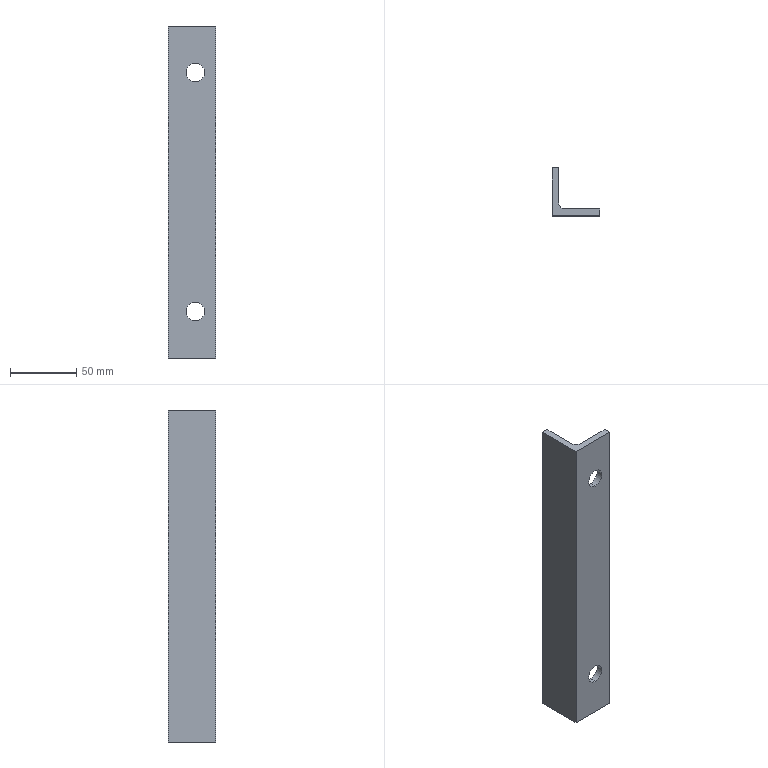Part | NX | features BREP 1 | 1 solid | 13 faces | box 36 x 36 x 250 mm | volume 83297 mm3 | plane 8 | cylinder 5 | commonest cylinder face diameters 14 x4 9 x1
STEP:
#1=CARTESIAN_POINT('',(20.5,0.,-97.));
#2=VERTEX_POINT('',#1);
#3=CARTESIAN_POINT('',(20.5,0.,-83.));
#4=VERTEX_POINT('',#3);
#5=CARTESIAN_POINT('',(20.5,0.,-90.));
#6=DIRECTION('',(0.,1.,0.));
#7=DIRECTION('',(0.,0.,-1.));
#8=AXIS2_PLACEMENT_3D('',#5,#6,#7);
#9=CIRCLE('',#8,7.);
#10=EDGE_CURVE('',#2,#4,#9,.T.);
#11=ORIENTED_EDGE('',*,*,#10,.F.);
#12=CARTESIAN_POINT('',(20.5,5.,-97.));
#13=VERTEX_POINT('',#12);
#14=CARTESIAN_POINT('',(20.5,0.,-97.));
#15=DIRECTION('',(0.,1.,0.));
#16=VECTOR('',#15,1000.);
#17=LINE('',#14,#16);
#18=EDGE_CURVE('',#2,#13,#17,.T.);
#19=ORIENTED_EDGE('',*,*,#18,.T.);
#20=CARTESIAN_POINT('',(20.5,5.,-83.));
#21=VERTEX_POINT('',#20);
#22=CARTESIAN_POINT('',(20.5,5.,-90.));
#23=DIRECTION('',(0.,1.,0.));
#24=DIRECTION('',(0.,0.,-1.));
#25=AXIS2_PLACEMENT_3D('',#22,#23,#24);
#26=CIRCLE('',#25,7.);
#27=EDGE_CURVE('',#13,#21,#26,.T.);
#28=ORIENTED_EDGE('',*,*,#27,.T.);
#29=CARTESIAN_POINT('',(20.5,0.,-83.));
#30=DIRECTION('',(0.,1.,0.));
#31=VECTOR('',#30,1000.);
#32=LINE('',#29,#31);
#33=EDGE_CURVE('',#4,#21,#32,.T.);
#34=ORIENTED_EDGE('',*,*,#33,.F.);
#35=EDGE_LOOP('',(#11,#19,#28,#34));
#36=FACE_BOUND('',#35,.T.);
#37=CARTESIAN_POINT('',(20.5,0.,-90.));
#38=DIRECTION('',(0.,1.,0.));
#39=DIRECTION('',(0.,0.,-1.));
#40=AXIS2_PLACEMENT_3D('',#37,#38,#39);
#41=CYLINDRICAL_SURFACE('',#40,7.);
#42=ADVANCED_FACE('',(#36),#41,.F.);
#43=CARTESIAN_POINT('',(20.5,0.,83.));
#44=VERTEX_POINT('',#43);
#45=CARTESIAN_POINT('',(20.5,0.,97.));
#46=VERTEX_POINT('',#45);
#47=CARTESIAN_POINT('',(20.5,0.,90.));
#48=DIRECTION('',(0.,1.,0.));
#49=DIRECTION('',(0.,0.,1.));
#50=AXIS2_PLACEMENT_3D('',#47,#48,#49);
#51=CIRCLE('',#50,7.);
#52=EDGE_CURVE('',#44,#46,#51,.T.);
#53=ORIENTED_EDGE('',*,*,#52,.F.);
#54=CARTESIAN_POINT('',(20.5,5.,83.));
#55=VERTEX_POINT('',#54);
#56=CARTESIAN_POINT('',(20.5,0.,83.));
#57=DIRECTION('',(0.,1.,0.));
#58=VECTOR('',#57,1000.);
#59=LINE('',#56,#58);
#60=EDGE_CURVE('',#44,#55,#59,.T.);
#61=ORIENTED_EDGE('',*,*,#60,.T.);
#62=CARTESIAN_POINT('',(20.5,5.,97.));
#63=VERTEX_POINT('',#62);
#64=CARTESIAN_POINT('',(20.5,5.,90.));
#65=DIRECTION('',(0.,1.,0.));
#66=DIRECTION('',(0.,0.,1.));
#67=AXIS2_PLACEMENT_3D('',#64,#65,#66);
#68=CIRCLE('',#67,7.);
#69=EDGE_CURVE('',#55,#63,#68,.T.);
#70=ORIENTED_EDGE('',*,*,#69,.T.);
#71=CARTESIAN_POINT('',(20.5,0.,97.));
#72=DIRECTION('',(0.,1.,0.));
#73=VECTOR('',#72,1000.);
#74=LINE('',#71,#73);
#75=EDGE_CURVE('',#46,#63,#74,.T.);
#76=ORIENTED_EDGE('',*,*,#75,.F.);
#77=EDGE_LOOP('',(#53,#61,#70,#76));
#78=FACE_BOUND('',#77,.T.);
#79=CARTESIAN_POINT('',(20.5,0.,90.));
#80=DIRECTION('',(0.,1.,0.));
#81=DIRECTION('',(0.,0.,-1.));
#82=AXIS2_PLACEMENT_3D('',#79,#80,#81);
#83=CYLINDRICAL_SURFACE('',#82,7.);
#84=ADVANCED_FACE('',(#78),#83,.F.);
#85=CARTESIAN_POINT('',(36.,0.,-125.));
#86=VERTEX_POINT('',#85);
#87=CARTESIAN_POINT('',(36.,5.,-125.));
#88=VERTEX_POINT('',#87);
#89=CARTESIAN_POINT('',(36.,5.,-125.));
#90=DIRECTION('',(0.,1.,0.));
#91=VECTOR('',#90,1000.);
#92=LINE('',#89,#91);
#93=EDGE_CURVE('',#86,#88,#92,.T.);
#94=ORIENTED_EDGE('',*,*,#93,.T.);
#95=CARTESIAN_POINT('',(36.,5.,125.));
#96=VERTEX_POINT('',#95);
#97=CARTESIAN_POINT('',(36.,5.,125.));
#98=DIRECTION('',(0.,0.,-1.));
#99=VECTOR('',#98,1000.);
#100=LINE('',#97,#99);
#101=EDGE_CURVE('',#96,#88,#100,.T.);
#102=ORIENTED_EDGE('',*,*,#101,.F.);
#103=CARTESIAN_POINT('',(36.,0.,125.));
#104=VERTEX_POINT('',#103);
#105=CARTESIAN_POINT('',(36.,5.,125.));
#106=DIRECTION('',(0.,1.,0.));
#107=VECTOR('',#106,1000.);
#108=LINE('',#105,#107);
#109=EDGE_CURVE('',#104,#96,#108,.T.);
#110=ORIENTED_EDGE('',*,*,#109,.F.);
#111=CARTESIAN_POINT('',(36.,0.,125.));
#112=DIRECTION('',(0.,0.,-1.));
#113=VECTOR('',#112,1000.);
#114=LINE('',#111,#113);
#115=EDGE_CURVE('',#104,#86,#114,.T.);
#116=ORIENTED_EDGE('',*,*,#115,.T.);
#117=EDGE_LOOP('',(#94,#102,#110,#116));
#118=FACE_BOUND('',#117,.T.);
#119=CARTESIAN_POINT('',(36.,5.,125.));
#120=DIRECTION('',(-1.,0.,0.));
#121=DIRECTION('',(0.,0.,-1.));
#122=AXIS2_PLACEMENT_3D('',#119,#120,#121);
#123=PLANE('',#122);
#124=ADVANCED_FACE('',(#118),#123,.F.);
#125=CARTESIAN_POINT('',(20.5,5.,-90.));
#126=DIRECTION('',(0.,1.,0.));
#127=DIRECTION('',(0.,0.,-1.));
#128=AXIS2_PLACEMENT_3D('',#125,#126,#127);
#129=CIRCLE('',#128,7.);
#130=EDGE_CURVE('',#21,#13,#129,.T.);
#131=ORIENTED_EDGE('',*,*,#130,.F.);
#132=ORIENTED_EDGE('',*,*,#27,.F.);
#133=EDGE_LOOP('',(#131,#132));
#134=FACE_BOUND('',#133,.T.);
#135=CARTESIAN_POINT('',(20.5,5.,90.));
#136=DIRECTION('',(0.,1.,0.));
#137=DIRECTION('',(0.,0.,1.));
#138=AXIS2_PLACEMENT_3D('',#135,#136,#137);
#139=CIRCLE('',#138,7.);
#140=EDGE_CURVE('',#63,#55,#139,.T.);
#141=ORIENTED_EDGE('',*,*,#140,.F.);
#142=ORIENTED_EDGE('',*,*,#69,.F.);
#143=EDGE_LOOP('',(#141,#142));
#144=FACE_BOUND('',#143,.T.);
#145=CARTESIAN_POINT('',(9.5,5.,-125.));
#146=VERTEX_POINT('',#145);
#147=CARTESIAN_POINT('',(9.5,5.,-125.));
#148=DIRECTION('',(-1.,0.,0.));
#149=VECTOR('',#148,1000.);
#150=LINE('',#147,#149);
#151=EDGE_CURVE('',#88,#146,#150,.T.);
#152=ORIENTED_EDGE('',*,*,#151,.T.);
#153=CARTESIAN_POINT('',(9.5,5.,125.));
#154=VERTEX_POINT('',#153);
#155=CARTESIAN_POINT('',(9.5,5.,125.));
#156=DIRECTION('',(0.,0.,-1.));
#157=VECTOR('',#156,1000.);
#158=LINE('',#155,#157);
#159=EDGE_CURVE('',#154,#146,#158,.T.);
#160=ORIENTED_EDGE('',*,*,#159,.F.);
#161=CARTESIAN_POINT('',(9.5,5.,125.));
#162=DIRECTION('',(-1.,0.,0.));
#163=VECTOR('',#162,1000.);
#164=LINE('',#161,#163);
#165=EDGE_CURVE('',#96,#154,#164,.T.);
#166=ORIENTED_EDGE('',*,*,#165,.F.);
#167=ORIENTED_EDGE('',*,*,#101,.T.);
#168=EDGE_LOOP('',(#152,#160,#166,#167));
#169=FACE_BOUND('',#168,.T.);
#170=CARTESIAN_POINT('',(9.5,5.,125.));
#171=DIRECTION('',(0.,-1.,0.));
#172=DIRECTION('',(0.,0.,1.));
#173=AXIS2_PLACEMENT_3D('',#170,#171,#172);
#174=PLANE('',#173);
#175=ADVANCED_FACE('',(#134,#144,#169),#174,.F.);
#176=CARTESIAN_POINT('',(5.,9.5,-125.));
#177=VERTEX_POINT('',#176);
#178=CARTESIAN_POINT('',(9.5,9.5,-125.));
#179=DIRECTION('',(0.,0.,-1.));
#180=DIRECTION('',(1.,0.,0.));
#181=AXIS2_PLACEMENT_3D('',#178,#179,#180);
#182=CIRCLE('',#181,4.5);
#183=EDGE_CURVE('',#146,#177,#182,.T.);
#184=ORIENTED_EDGE('',*,*,#183,.T.);
#185=CARTESIAN_POINT('',(5.,9.5,125.));
#186=VERTEX_POINT('',#185);
#187=CARTESIAN_POINT('',(5.,9.5,125.));
#188=DIRECTION('',(0.,0.,-1.));
#189=VECTOR('',#188,1000.);
#190=LINE('',#187,#189);
#191=EDGE_CURVE('',#186,#177,#190,.T.);
#192=ORIENTED_EDGE('',*,*,#191,.F.);
#193=CARTESIAN_POINT('',(9.5,9.5,125.));
#194=DIRECTION('',(0.,0.,-1.));
#195=DIRECTION('',(1.,0.,0.));
#196=AXIS2_PLACEMENT_3D('',#193,#194,#195);
#197=CIRCLE('',#196,4.5);
#198=EDGE_CURVE('',#154,#186,#197,.T.);
#199=ORIENTED_EDGE('',*,*,#198,.F.);
#200=ORIENTED_EDGE('',*,*,#159,.T.);
#201=EDGE_LOOP('',(#184,#192,#199,#200));
#202=FACE_BOUND('',#201,.T.);
#203=CARTESIAN_POINT('',(9.5,9.5,125.));
#204=DIRECTION('',(0.,0.,-1.));
#205=DIRECTION('',(1.,0.,0.));
#206=AXIS2_PLACEMENT_3D('',#203,#204,#205);
#207=CYLINDRICAL_SURFACE('',#206,4.5);
#208=ADVANCED_FACE('',(#202),#207,.F.);
#209=CARTESIAN_POINT('',(5.,36.,-125.));
#210=VERTEX_POINT('',#209);
#211=CARTESIAN_POINT('',(5.,36.,-125.));
#212=DIRECTION('',(0.,1.,0.));
#213=VECTOR('',#212,1000.);
#214=LINE('',#211,#213);
#215=EDGE_CURVE('',#177,#210,#214,.T.);
#216=ORIENTED_EDGE('',*,*,#215,.T.);
#217=CARTESIAN_POINT('',(5.,36.,125.));
#218=VERTEX_POINT('',#217);
#219=CARTESIAN_POINT('',(5.,36.,125.));
#220=DIRECTION('',(0.,0.,-1.));
#221=VECTOR('',#220,1000.);
#222=LINE('',#219,#221);
#223=EDGE_CURVE('',#218,#210,#222,.T.);
#224=ORIENTED_EDGE('',*,*,#223,.F.);
#225=CARTESIAN_POINT('',(5.,36.,125.));
#226=DIRECTION('',(0.,1.,0.));
#227=VECTOR('',#226,1000.);
#228=LINE('',#225,#227);
#229=EDGE_CURVE('',#186,#218,#228,.T.);
#230=ORIENTED_EDGE('',*,*,#229,.F.);
#231=ORIENTED_EDGE('',*,*,#191,.T.);
#232=EDGE_LOOP('',(#216,#224,#230,#231));
#233=FACE_BOUND('',#232,.T.);
#234=CARTESIAN_POINT('',(5.,36.,125.));
#235=DIRECTION('',(-1.,0.,0.));
#236=DIRECTION('',(0.,0.,-1.));
#237=AXIS2_PLACEMENT_3D('',#234,#235,#236);
#238=PLANE('',#237);
#239=ADVANCED_FACE('',(#233),#238,.F.);
#240=CARTESIAN_POINT('',(0.,36.,-125.));
#241=VERTEX_POINT('',#240);
#242=CARTESIAN_POINT('',(0.,36.,-125.));
#243=DIRECTION('',(-1.,0.,0.));
#244=VECTOR('',#243,1000.);
#245=LINE('',#242,#244);
#246=EDGE_CURVE('',#210,#241,#245,.T.);
#247=ORIENTED_EDGE('',*,*,#246,.T.);
#248=CARTESIAN_POINT('',(0.,36.,125.));
#249=VERTEX_POINT('',#248);
#250=CARTESIAN_POINT('',(0.,36.,125.));
#251=DIRECTION('',(0.,0.,-1.));
#252=VECTOR('',#251,1000.);
#253=LINE('',#250,#252);
#254=EDGE_CURVE('',#249,#241,#253,.T.);
#255=ORIENTED_EDGE('',*,*,#254,.F.);
#256=CARTESIAN_POINT('',(0.,36.,125.));
#257=DIRECTION('',(-1.,0.,0.));
#258=VECTOR('',#257,1000.);
#259=LINE('',#256,#258);
#260=EDGE_CURVE('',#218,#249,#259,.T.);
#261=ORIENTED_EDGE('',*,*,#260,.F.);
#262=ORIENTED_EDGE('',*,*,#223,.T.);
#263=EDGE_LOOP('',(#247,#255,#261,#262));
#264=FACE_BOUND('',#263,.T.);
#265=CARTESIAN_POINT('',(0.,36.,125.));
#266=DIRECTION('',(0.,-1.,0.));
#267=DIRECTION('',(0.,0.,1.));
#268=AXIS2_PLACEMENT_3D('',#265,#266,#267);
#269=PLANE('',#268);
#270=ADVANCED_FACE('',(#264),#269,.F.);
#271=CARTESIAN_POINT('',(0.,0.,-125.));
#272=VERTEX_POINT('',#271);
#273=CARTESIAN_POINT('',(0.,0.,-125.));
#274=DIRECTION('',(0.,-1.,0.));
#275=VECTOR('',#274,1000.);
#276=LINE('',#273,#275);
#277=EDGE_CURVE('',#241,#272,#276,.T.);
#278=ORIENTED_EDGE('',*,*,#277,.T.);
#279=CARTESIAN_POINT('',(0.,0.,125.));
#280=VERTEX_POINT('',#279);
#281=CARTESIAN_POINT('',(0.,0.,125.));
#282=DIRECTION('',(0.,0.,-1.));
#283=VECTOR('',#282,1000.);
#284=LINE('',#281,#283);
#285=EDGE_CURVE('',#280,#272,#284,.T.);
#286=ORIENTED_EDGE('',*,*,#285,.F.);
#287=CARTESIAN_POINT('',(0.,0.,125.));
#288=DIRECTION('',(0.,-1.,0.));
#289=VECTOR('',#288,1000.);
#290=LINE('',#287,#289);
#291=EDGE_CURVE('',#249,#280,#290,.T.);
#292=ORIENTED_EDGE('',*,*,#291,.F.);
#293=ORIENTED_EDGE('',*,*,#254,.T.);
#294=EDGE_LOOP('',(#278,#286,#292,#293));
#295=FACE_BOUND('',#294,.T.);
#296=CARTESIAN_POINT('',(0.,0.,125.));
#297=DIRECTION('',(1.,0.,0.));
#298=DIRECTION('',(0.,0.,1.));
#299=AXIS2_PLACEMENT_3D('',#296,#297,#298);
#300=PLANE('',#299);
#301=ADVANCED_FACE('',(#295),#300,.F.);
#302=CARTESIAN_POINT('',(20.5,0.,-90.));
#303=DIRECTION('',(0.,1.,0.));
#304=DIRECTION('',(0.,0.,-1.));
#305=AXIS2_PLACEMENT_3D('',#302,#303,#304);
#306=CIRCLE('',#305,7.);
#307=EDGE_CURVE('',#4,#2,#306,.T.);
#308=ORIENTED_EDGE('',*,*,#307,.T.);
#309=ORIENTED_EDGE('',*,*,#10,.T.);
#310=EDGE_LOOP('',(#308,#309));
#311=FACE_BOUND('',#310,.T.);
#312=CARTESIAN_POINT('',(20.5,0.,90.));
#313=DIRECTION('',(0.,1.,0.));
#314=DIRECTION('',(0.,0.,1.));
#315=AXIS2_PLACEMENT_3D('',#312,#313,#314);
#316=CIRCLE('',#315,7.);
#317=EDGE_CURVE('',#46,#44,#316,.T.);
#318=ORIENTED_EDGE('',*,*,#317,.T.);
#319=ORIENTED_EDGE('',*,*,#52,.T.);
#320=EDGE_LOOP('',(#318,#319));
#321=FACE_BOUND('',#320,.T.);
#322=CARTESIAN_POINT('',(36.,0.,-125.));
#323=DIRECTION('',(1.,0.,0.));
#324=VECTOR('',#323,1000.);
#325=LINE('',#322,#324);
#326=EDGE_CURVE('',#272,#86,#325,.T.);
#327=ORIENTED_EDGE('',*,*,#326,.T.);
#328=ORIENTED_EDGE('',*,*,#115,.F.);
#329=CARTESIAN_POINT('',(36.,0.,125.));
#330=DIRECTION('',(1.,0.,0.));
#331=VECTOR('',#330,1000.);
#332=LINE('',#329,#331);
#333=EDGE_CURVE('',#280,#104,#332,.T.);
#334=ORIENTED_EDGE('',*,*,#333,.F.);
#335=ORIENTED_EDGE('',*,*,#285,.T.);
#336=EDGE_LOOP('',(#327,#328,#334,#335));
#337=FACE_BOUND('',#336,.T.);
#338=CARTESIAN_POINT('',(36.,0.,125.));
#339=DIRECTION('',(0.,1.,0.));
#340=DIRECTION('',(0.,0.,-1.));
#341=AXIS2_PLACEMENT_3D('',#338,#339,#340);
#342=PLANE('',#341);
#343=ADVANCED_FACE('',(#311,#321,#337),#342,.F.);
#344=ORIENTED_EDGE('',*,*,#109,.T.);
#345=ORIENTED_EDGE('',*,*,#165,.T.);
#346=ORIENTED_EDGE('',*,*,#198,.T.);
#347=ORIENTED_EDGE('',*,*,#229,.T.);
#348=ORIENTED_EDGE('',*,*,#260,.T.);
#349=ORIENTED_EDGE('',*,*,#291,.T.);
#350=ORIENTED_EDGE('',*,*,#333,.T.);
#351=EDGE_LOOP('',(#344,#345,#346,#347,#348,#349,#350));
#352=FACE_BOUND('',#351,.T.);
#353=CARTESIAN_POINT('',(9.5,9.5,125.));
#354=DIRECTION('',(0.,0.,1.));
#355=DIRECTION('',(-1.,0.,0.));
#356=AXIS2_PLACEMENT_3D('',#353,#354,#355);
#357=PLANE('',#356);
#358=ADVANCED_FACE('',(#352),#357,.T.);
#359=ORIENTED_EDGE('',*,*,#93,.F.);
#360=ORIENTED_EDGE('',*,*,#326,.F.);
#361=ORIENTED_EDGE('',*,*,#277,.F.);
#362=ORIENTED_EDGE('',*,*,#246,.F.);
#363=ORIENTED_EDGE('',*,*,#215,.F.);
#364=ORIENTED_EDGE('',*,*,#183,.F.);
#365=ORIENTED_EDGE('',*,*,#151,.F.);
#366=EDGE_LOOP('',(#359,#360,#361,#362,#363,#364,#365));
#367=FACE_BOUND('',#366,.T.);
#368=CARTESIAN_POINT('',(9.5,9.5,-125.));
#369=DIRECTION('',(0.,0.,1.));
#370=DIRECTION('',(-1.,0.,0.));
#371=AXIS2_PLACEMENT_3D('',#368,#369,#370);
#372=PLANE('',#371);
#373=ADVANCED_FACE('',(#367),#372,.F.);
#374=ORIENTED_EDGE('',*,*,#60,.F.);
#375=ORIENTED_EDGE('',*,*,#317,.F.);
#376=ORIENTED_EDGE('',*,*,#75,.T.);
#377=ORIENTED_EDGE('',*,*,#140,.T.);
#378=EDGE_LOOP('',(#374,#375,#376,#377));
#379=FACE_BOUND('',#378,.T.);
#380=CARTESIAN_POINT('',(20.5,0.,90.));
#381=DIRECTION('',(0.,1.,0.));
#382=DIRECTION('',(0.,0.,-1.));
#383=AXIS2_PLACEMENT_3D('',#380,#381,#382);
#384=CYLINDRICAL_SURFACE('',#383,7.);
#385=ADVANCED_FACE('',(#379),#384,.F.);
#386=ORIENTED_EDGE('',*,*,#18,.F.);
#387=ORIENTED_EDGE('',*,*,#307,.F.);
#388=ORIENTED_EDGE('',*,*,#33,.T.);
#389=ORIENTED_EDGE('',*,*,#130,.T.);
#390=EDGE_LOOP('',(#386,#387,#388,#389));
#391=FACE_BOUND('',#390,.T.);
#392=CARTESIAN_POINT('',(20.5,0.,-90.));
#393=DIRECTION('',(0.,1.,0.));
#394=DIRECTION('',(0.,0.,-1.));
#395=AXIS2_PLACEMENT_3D('',#392,#393,#394);
#396=CYLINDRICAL_SURFACE('',#395,7.);
#397=ADVANCED_FACE('',(#391),#396,.F.);
#398=CLOSED_SHELL('',(#42,#84,#124,#175,#208,#239,#270,#301,#343,#358,#373,#385,#397));
#399=MANIFOLD_SOLID_BREP('',#398);
#400=(LENGTH_UNIT()NAMED_UNIT(*)SI_UNIT(.MILLI.,.METRE.));
#401=UNCERTAINTY_MEASURE_WITH_UNIT(LENGTH_MEASURE(0.00001),#400,'','');
#402=(NAMED_UNIT(*)PLANE_ANGLE_UNIT()SI_UNIT($,.RADIAN.));
#403=(NAMED_UNIT(*)SI_UNIT($,.STERADIAN.)SOLID_ANGLE_UNIT());
#404=(GEOMETRIC_REPRESENTATION_CONTEXT(3)GLOBAL_UNCERTAINTY_ASSIGNED_CONTEXT((#401))GLOBAL_UNIT_ASSIGNED_CONTEXT((#400,#402,#403))REPRESENTATION_CONTEXT('',''));
#405=ADVANCED_BREP_SHAPE_REPRESENTATION('',(#399),#404);